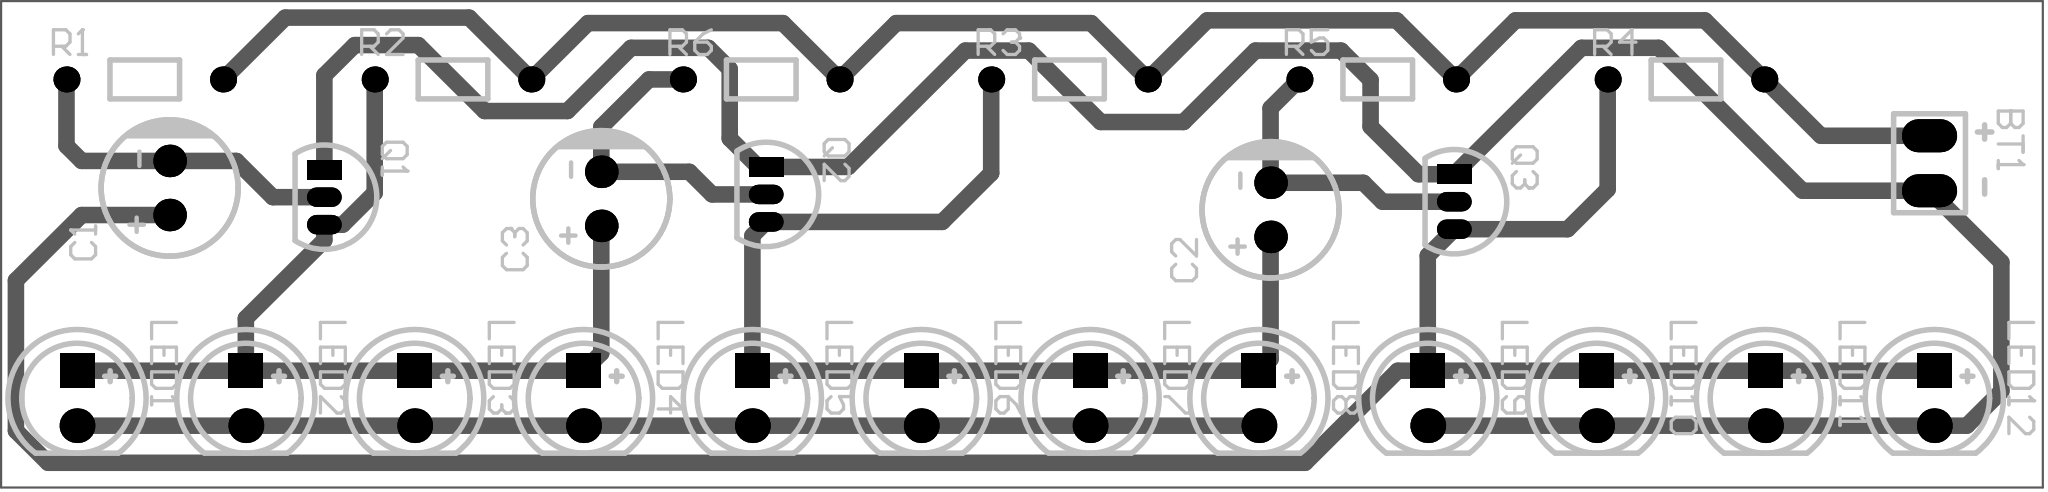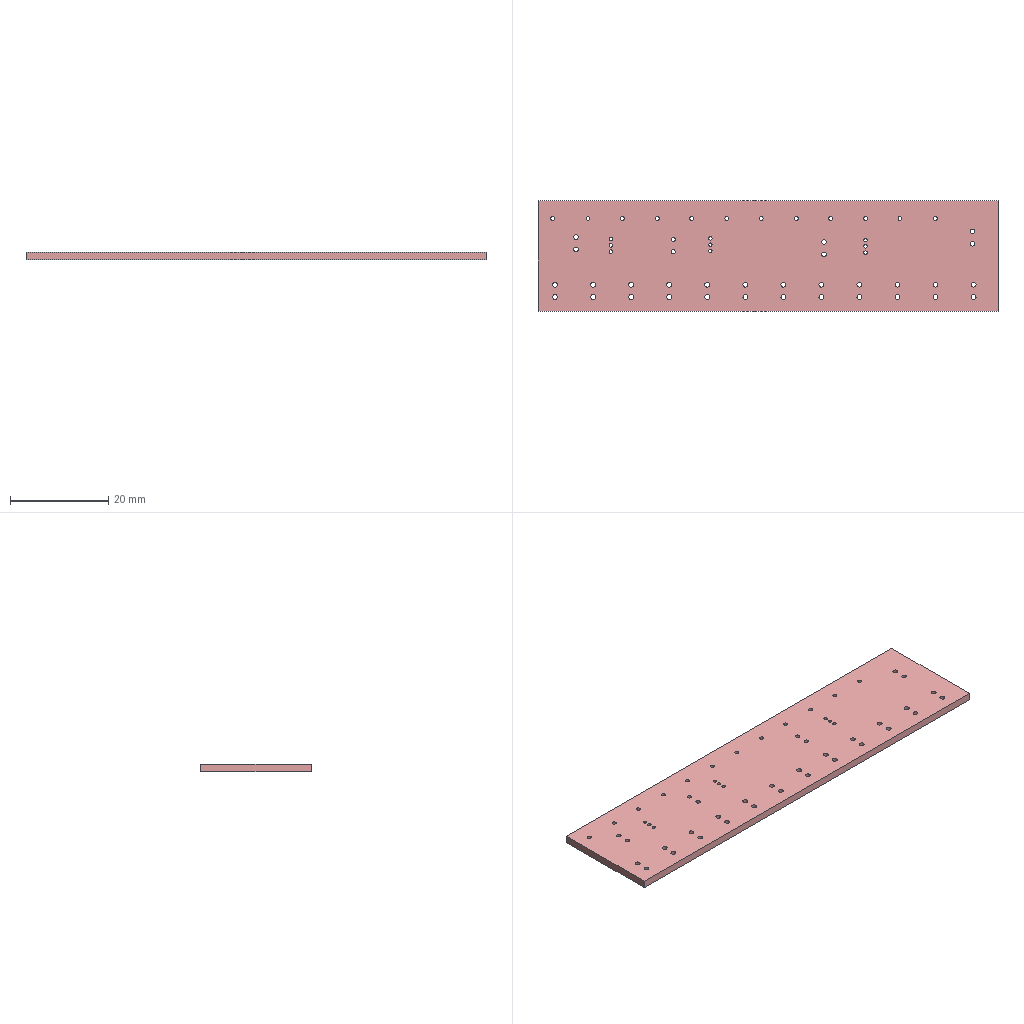Circuit board layout | Altium Designer | box 93.9 x 22.5 x 1.6 mm
Layer stack:
# Altium Designer layer stack of  (unit mm; dielectric type: 0 none, 1 core, 2 prepreg, 3 surface material)
index,name,kind,layer,copper_thickness_mm,dielectric_type,dielectric_thickness_mm,dielectric_material,dielectric_constant
0,Top Paste Mask Layer,other,,,,,,
1,Top Silkscreen Layer,other,,,,,,
2,Top Solder Mask Layer,dielectric,,,3,0.01,,3.3
3,Top Layer,copper,Top Layer,0.035,,,,
4,Dielectric1,dielectric,,,3,1.51,FR4,4.5
5,Bottom Layer,copper,Bottom Layer,0.035,,,,
6,Bottom Solder Mask Layer,dielectric,,,3,0.01,,3.3
7,Bottom Silkscreen Layer,other,,,,,,
8,Bottom Paste Mask Layer,other,,,,,,
# drill layer pairs: low layer,high layer
drill_pair,Top Layer,Bottom Layer
Part placement:
Designator,Comment,Layer,Footprint,Center-X(mm),Center-Y(mm),Rotation
BT1,9V battery wire clip Cu 100mm,TopLayer,BAT-TH_2P-9VBATTERY,164.846,91.186,270
C1,47uF,TopLayer,CAP-TH_BD6.3-P2.50-D0.5-FD,83.947,90.043,90
C2,47uF,TopLayer,CAP-TH_BD6.3-P2.50-D0.5-FD,134.554,89.034,90
C3,47uF,TopLayer,CAP-TH_BD6.3-P2.50-D0.5-FD,103.789,89.542,90
LED1,,TopLayer,LED-TH_5mm,79.689,80.328,270
LED2,,TopLayer,LED-TH_5mm,87.451,80.328,270
LED3,,TopLayer,LED-TH_5mm,95.212,80.328,270
LED4,,TopLayer,LED-TH_5mm,102.973,80.328,270
LED5,,TopLayer,LED-TH_5mm,110.735,80.328,270
LED6,,TopLayer,LED-TH_5mm,118.496,80.328,270
LED7,,TopLayer,LED-TH_5mm,126.258,80.328,270
LED8,,TopLayer,LED-TH_5mm,134.019,80.328,270
LED9,,TopLayer,LED-TH_5mm,141.781,80.328,270
LED10,,TopLayer,LED-TH_5mm,149.542,80.328,270
LED11,,TopLayer,LED-TH_5mm,157.304,80.328,270
LED12,,TopLayer,LED-TH_5mm,165.065,80.328,270
R1,9.1kΩ,TopLayer,Res_1/8W,82.804,95.059,0
R2,470,TopLayer,Res_1/8W,96.973,95.059,0
R3,470,TopLayer,Res_1/8W,125.312,95.059,0
R4,470,TopLayer,Res_1/8W,153.65,95.059,0
R5,10kΩ,TopLayer,Res_1/8W,139.481,95.059,0
R6,10kΩ,TopLayer,Res_1/8W,111.142,95.059,0
Q1,,TopLayer,S8050_TO_92,91.059,89.618,270
Q2,,TopLayer,S8050_TO_92,111.371,89.745,270
Q3,,TopLayer,S8050_TO_92,143.002,89.408,270
Pad and via stacks:
# Altium Designer via and pad stacks of  (unit mm). Each distinct definition once, with the count of objects using it.
# via: kind,start_layer,end_layer,hole_mm,diameter_mm,mode(0 simple;1 top-mid-bottom;2 full stack),diameter_per_layer,count,example_net
# pad: kind,layer,hole_mm,hole_type(0 round;1 square;2 slot),plating,top_size,top_shape(1 round;2 rect;3 octagon;9 rounded rect),mid_size,bottom_size,mode,footprint,size_per_layer,count,example
pad,Multi-Layer,0.9144,0,plated,1.524x2.54,1,1.524x2.54,1.524x2.54,0,BAT-TH_2P-9VBATTERY,,2,BT1.1
pad,Multi-Layer,0.9,0,plated,1.5x1.5,1,1.5x1.5,1.5x1.5,0,CAP-TH_BD6.3-P2.50-D0.5-FD,,6,C1.2
pad,Multi-Layer,1,0,plated,1.6x1.6,2,1.6x1.6,1.6x1.6,0,LED-TH_5mm,,12,LED1.1
pad,Multi-Layer,1,0,plated,1.6x1.6,1,1.6x1.6,1.6x1.6,0,LED-TH_5mm,,12,LED1.2
pad,Multi-Layer,0.8001,0,plated,1.199x1.199,1,1.199x1.199,1.199x1.199,0,Res_1/8W,,12,R1.1
pad,Multi-Layer,0.701,0,plated,0.8992x1.6,2,0.8992x1.6,0.8992x1.6,0,S8050_TO_92,,3,Q1.1
pad,Multi-Layer,0.701,0,plated,0.8992x1.6,1,0.8992x1.6,0.8992x1.6,0,S8050_TO_92,,6,Q1.2